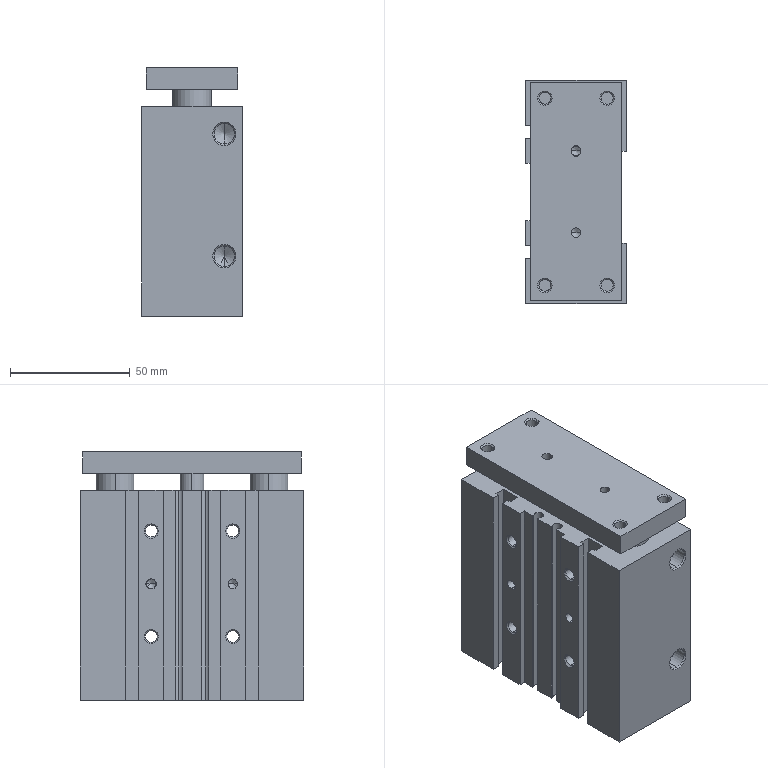Part | SolidWorks | 2 solids | 234 faces | box 42 x 93 x 103.5 mm | volume 316808 mm3 | cylinder 88 | plane 78 | cone 68 | commonest cylinder face diameters 4.917 x24 4 x18 5.4 x8 8.566 x8 9.5 x8 16 x8